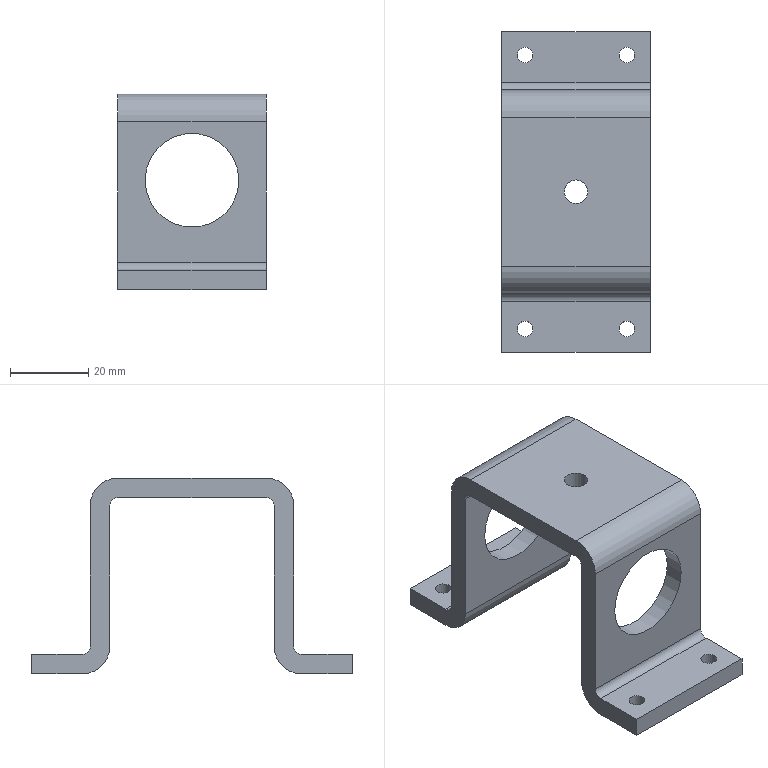Part | STEP file | 1-46.1 | 1 solid | 29 faces | box 38 x 82 x 50 mm | volume 26296 mm3 | cylinder 15 | plane 14 | commonest cylinder face diameters 4 x8 14 x4 24 x2 6 x1